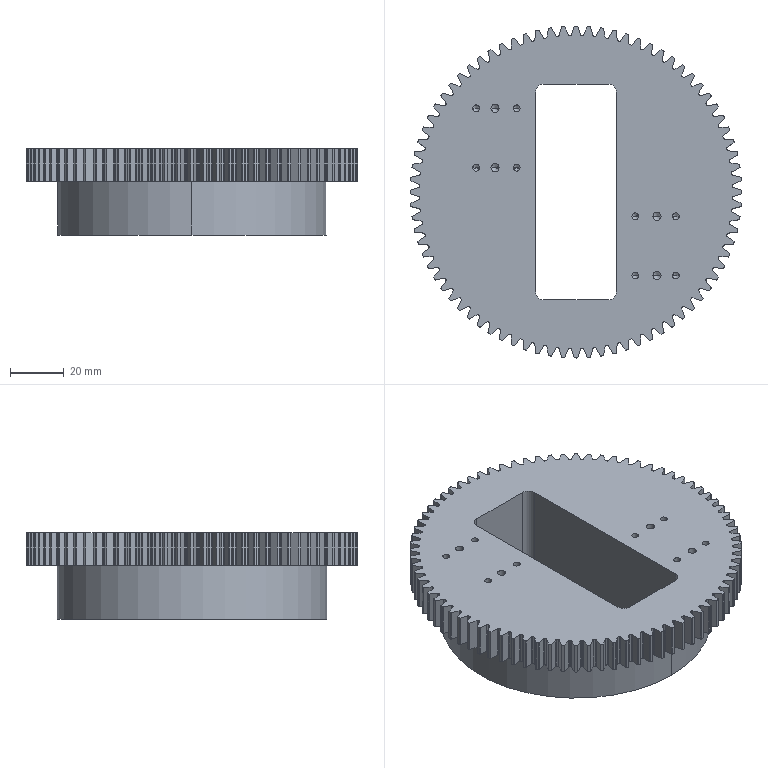Part | NX | features BREP 1 | 1 solid | 830 faces | box 123 x 123 x 32 mm | volume 210252 mm3 | cylinder 607 | plane 167 | cone 56 | commonest cylinder face diameters 0.75 x194 0.4 x190 123 x81 116.25 x80 5 x24 2.5 x16